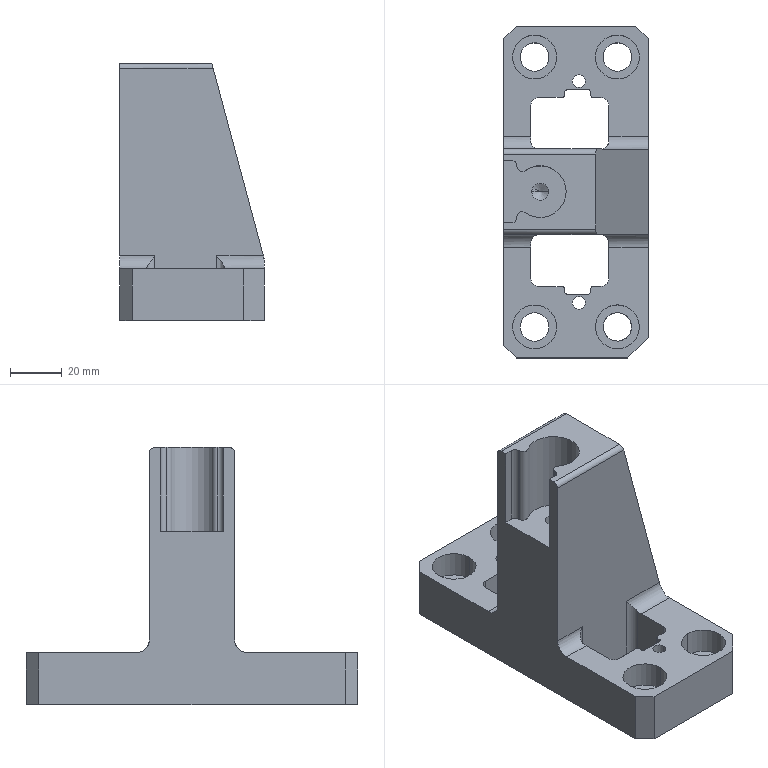Part | STEP file | 1_id682_x_t | 1 solid | 89 faces | box 56 x 128.26 x 99.32 mm | volume 209835 mm3 | cylinder 49 | plane 38 | cone 2 | commonest cylinder face diameters 2 x8 6.1 x8 11 x8 17 x8 4 x6 5 x4